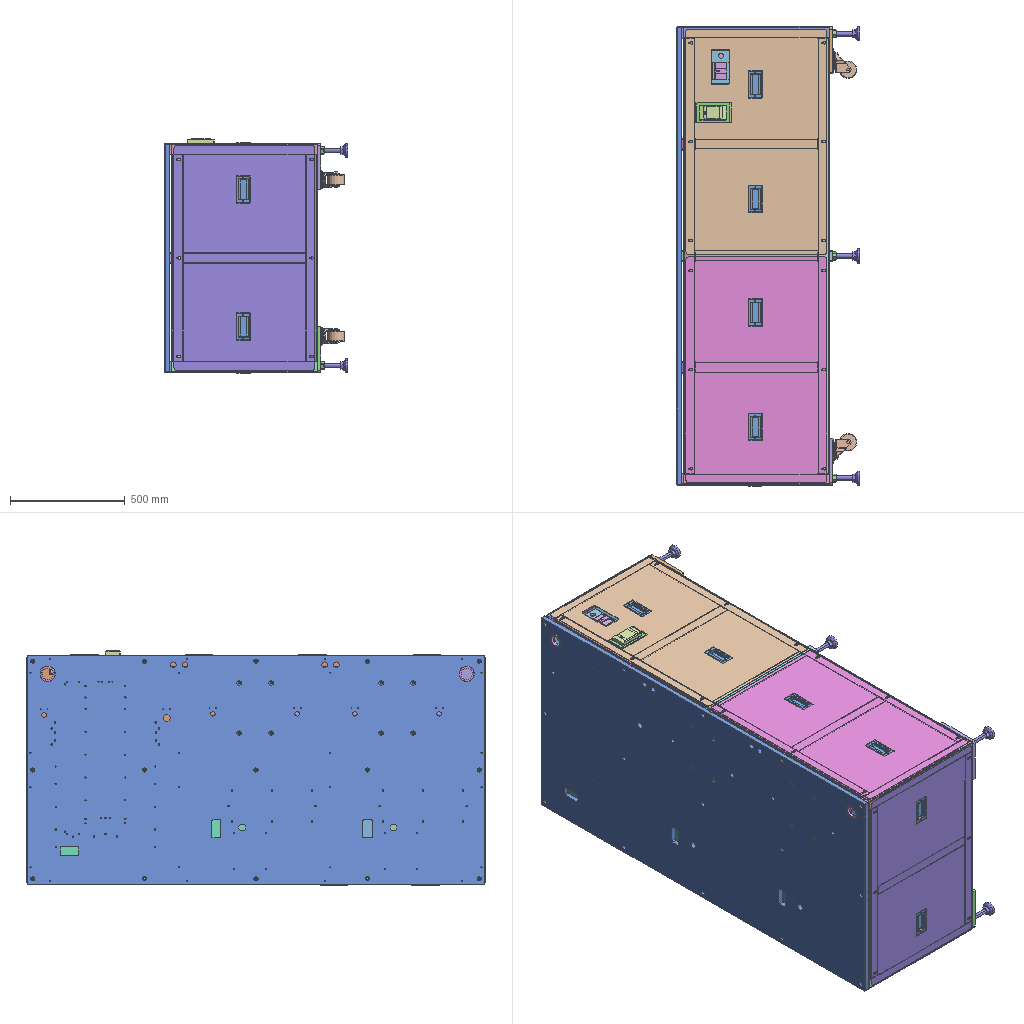Assembly | SolidWorks | 34 different items | 81 placed | box 804 x 2008 x 1025 mm
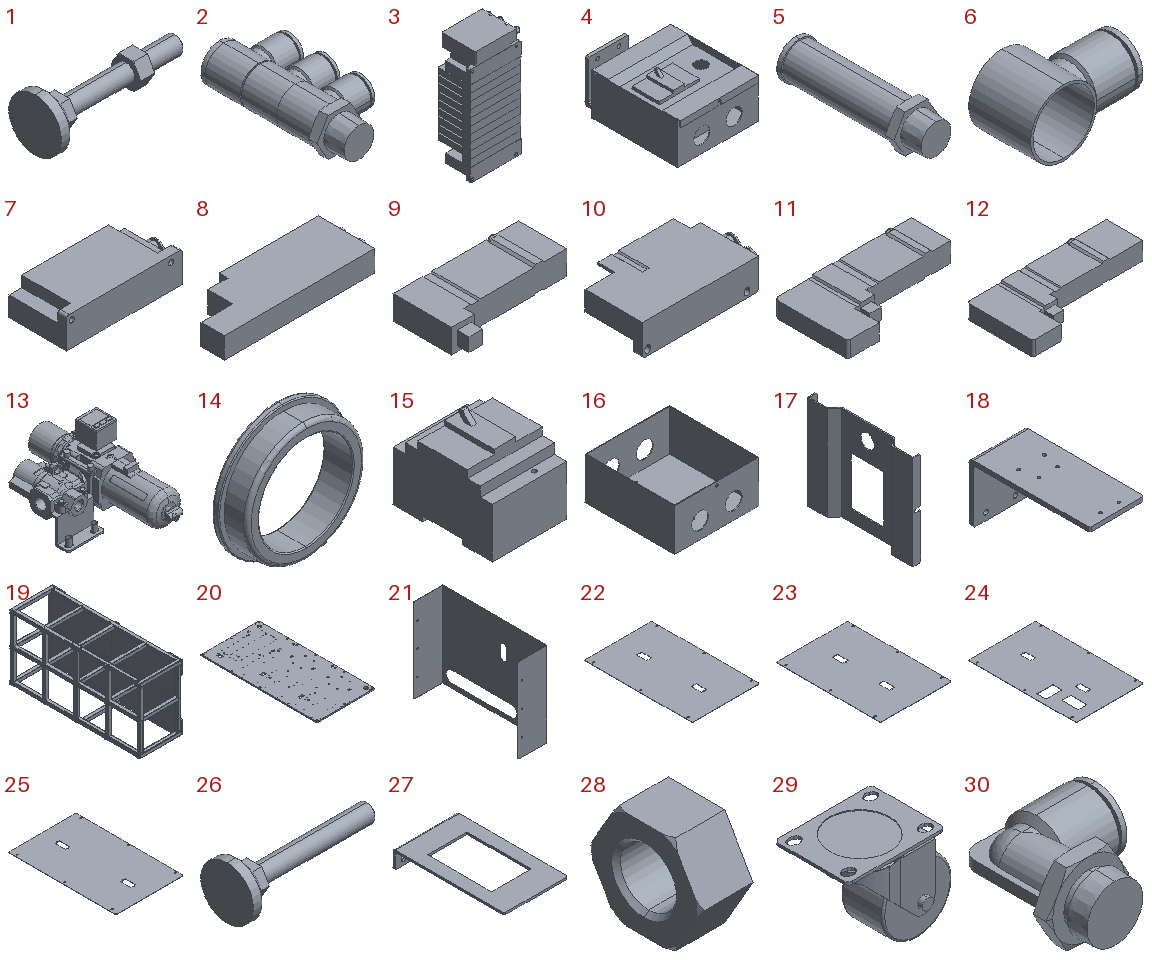Parts list (item | name | quantity | parent item | size | volume | features):
1 | (subassembly) | x6 | - | 161 x 60 x 60 mm | 104364 mm3 | -
2 | (subassembly) | x1 | - | 37.824 x 76.6 x 21 mm | 29874 mm3 | features RefAxis 3
3 | (subassembly) | x1 | - | - | 1754450 mm3 | -
4 | (subassembly) | x1 | - | 150 x 195.998 x 89.507 mm | 688254 mm3 | -
5 | - | x1 | in 2 | 24.249 x 76.6 x 21 mm | 21613 mm3 | features RefAxis 3, BaseBody 1, MoveFace 1
6 | - | x3 | in 2 | 36 x 19.2 x 20.6 mm | 2754 mm3 | features RefAxis 3, BaseBody 1
7 | - | x1 | in 3 | 121.7 x 73.2 x 30 mm | 182258 mm3 | features BaseBody 1
8 | - | x10 | in 3 | 117.6 x 42.6 x 16 mm | 66009 mm3 | features BaseBody 1
9 | - | x1 | in 3 | 78.8 x 44.194 x 18.1 mm | 37684 mm3 | features BaseBody 1
10 | - | x1 | in 3 | 121.7 x 73.2 x 30.5 mm | 162899 mm3 | features BaseBody 1
11 | - | x3 | in 3 | 103.4 x 55.58 x 18.1 mm | 53626 mm3 | features BaseBody 1
12 | - | x6 | in 3 | 116.6 x 55.58 x 18.1 mm | 59586 mm3 | features BaseBody 1
13 | - | x1 | - | - | - | features RefSurface 14, ExtruRefSurface 1
14 | - | x2 | - | 67 x 15.5 x 67 mm | 18291 mm3 | features Fillet 3, ICE 2, Extrusion 1
15 | - | x1 | in 4 | 74.7 x 99.6 x 82.007 mm | 445552 mm3 | features ICE 5, Extrusion 1, Fillet 1, HoleWzd 1
16 | - | x1 | in 4 | 150 x 163 x 75 mm | 99364 mm3 | features HoleWzd 3, ICE 2, Extrusion 1, Shell 1
17 | - | x1 | in 4 | 13.5 x 164.498 x 147 mm | 37040 mm3 | features ICE 4, Chamfer 1, ExtruThin 1, MirrorPattern 1
18 | - | x1 | in 4 | 75 x 165 x 80 mm | 106298 mm3 | features HoleWzd 3, Fillet 2, Chamfer 1, Extrusion 1, Shell 1
19 | - | x1 | - | 660 x 2000 x 1000 mm | 17994885 mm3 | features Fillet 21, HoleWzd 17, WeldCornerFeat 11, ICE 6, Chamfer 4, WeldMemberFeat 3, 3DProfileFeature 1, MoveFace 1, WeldmentFeature 1
20 | - | x1 | - | 1000 x 2000 x 20 mm | 39453468 mm3 | features HoleWzd 18, Cut 5, Chamfer 2, Extrusion 1, Fillet 1, ICE 1, MirrorPattern 1
21 | - | x1 | - | 150 x 533 x 430 mm | 664905 mm3 | features Cut 2, HoleWzd 2, Fillet 1, FlatPattern 1, ICE 1, LPattern 1, SMBaseFlange 1, SheetMetal 1
22 | - | x1 | - | 615 x 985 x 2 mm | 1193141 mm3 | features ICE 4, Extrusion 1, Fillet 1, LPattern 1
23 | - | x1 | - | 615 x 900 x 2 mm | 1088591 mm3 | features ICE 4, Extrusion 1, Fillet 1, HoleWzd 1, LPattern 1
24 | - | x1 | - | 615 x 983 x 2 mm | 1141777 mm3 | features ICE 6, Fillet 2, Extrusion 1, LPattern 1
25 | - | x2 | - | 615 x 980 x 2 mm | 1186991 mm3 | features ICE 4, Extrusion 1, Fillet 1, LPattern 1
26 | - | x6 | in 1 | 161 x 60 x 60 mm | 95763 mm3 | features RefAxis 9, 3DProfileFeature 3, ICE 1, Revolution 1
27 | - | x1 | - | 90 x 158 x 25 mm | 32642 mm3 | features Fillet 2, ICE 2, EdgeFlange 1, FlatPattern 1, SMBaseFlange 1, SheetMetal 1
28 | - | x6 | in 1 | 16 x 34.641 x 30 mm | 8601 mm3 | features RefAxis 3, 3DProfileFeature 1, ICE 1, Revolution 1
29 | - | x4 | - | 130 x 80 x 106 mm | 293823 mm3 | features ICE 12, Fillet 4, Revolution 2, Extrusion 1
30 | - | x1 | - | 33.624 x 36.35 x 21 mm | 9019 mm3 | features BaseBody 1
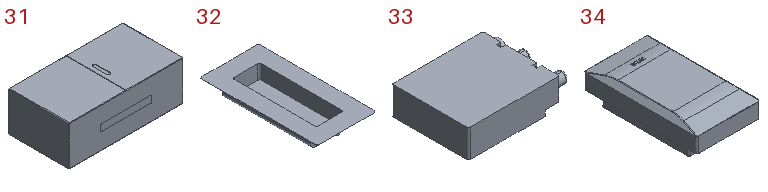31 | - | x1 | - | 1000 x 530 x 350 mm | 185406118 mm3 | features ICE 3, Fillet 2, Cut 1, Extrusion 1
32 | - | x10 | - | 60 x 120 x 15 mm | 28231 mm3 | features RefAxis 6, ICE 4, 3DProfileFeature 2, Revolution 2, Extrusion 1
33 | - | x1 | in 3 | 102.4 x 76.5 x 28.2 mm | 193130 mm3 | features BaseBody 1
34 | - | x1 | - | 65 x 116 x 32 mm | 202668 mm3 | features Fillet 5, Chamfer 3, ICE 2, Emboss 1, Extrusion 1
Mates (type | each side: item.copy, entity, surface, feature):
In the top assembly
Coincident | 19.1 face plane Boss-Extrude7 | 20.1 face plane Boss-Extrude1
Coincident | 19.1 face plane Structural Member6 | 20.1 face plane Boss-Extrude1
Concentric | 19.1 face cylinder M20 Tapped Hole1 | 26.1 face cylinder Revolve1
Coincident | 19.1 face plane Boss-Extrude2 | 28.1 face plane Revolve1
Concentric | 19.1 face cylinder M20 Tapped Hole1 | 26.2 face cylinder Revolve1
Coincident | 19.1 face plane Boss-Extrude2 | 28.2 face plane Revolve1
Concentric | 19.1 face cylinder M20 Tapped Hole2 | 26.3 face cylinder Revolve1
Coincident | 19.1 face plane Boss-Extrude25 | 28.3 face plane Revolve1
Concentric | 19.1 face cylinder M20 Tapped Hole2 | 26.4 face cylinder Revolve1
Coincident | 19.1 face plane Boss-Extrude25 | 28.4 face plane Revolve1
Concentric | 19.1 face cylinder M20 Tapped Hole1 | 26.5 face cylinder Revolve1
Coincident | 19.1 face plane Boss-Extrude2 | 28.5 face plane Revolve1
Concentric | 19.1 face cylinder M20 Tapped Hole1 | 26.6 face cylinder Revolve1
Coincident | 19.1 face plane Boss-Extrude2 | 28.6 face plane Revolve1
Concentric | 19.1 face cylinder M8 Tapped Hole1 | 29.1 face cylinder Cut-Extrude10 | 2 times
Coincident | 19.1 face plane Boss-Extrude2 | 29.1 face plane Boss-Extrude1
Concentric | 19.1 face cylinder M8 Tapped Hole1 | 29.2 face cylinder Cut-Extrude10 | 2 times
Coincident | 19.1 face plane Boss-Extrude2 | 29.2 face plane Boss-Extrude1
Concentric | 19.1 face cylinder M8 Tapped Hole1 | 29.3 face cylinder Cut-Extrude10 | 2 times
Coincident | 19.1 face plane Boss-Extrude2 | 29.3 face plane Boss-Extrude1
Concentric | 19.1 face cylinder M8 Tapped Hole1 | 29.4 face cylinder Cut-Extrude10 | 2 times
Coincident | 19.1 face plane Boss-Extrude2 | 29.4 face plane Boss-Extrude1
Coincident | 19.1 face plane Structural Member9 | 20.1 face plane Boss-Extrude1
Coincident | 19.1 face plane Structural Member5 | 25.1 face plane Boss-Extrude1
DistanceDim | 19.1 face plane Structural Member5 | 25.1 face plane Boss-Extrude1
DistanceDim | 25.1 face plane Boss-Extrude1 | 19.1 face plane Structural Member9
Coincident | 19.1 face plane Structural Member6 | 21.1 face plane Base-Flange1
DistanceDim | 21.1 face plane Base-Flange1 | 19.1 face plane Structural Member6
Coincident | 19.1 face plane Structural Member6 | 18.1 face plane Boss-Extrude1
DistanceDim | 17.1 face plane Extrude-Thin1 | 19.1 face plane Structural Member6
Coincident | 19.1 face plane Structural Member5 | 22.1 face plane Boss-Extrude1
DistanceDim | 19.1 face plane Structural Member5 | 22.1 face plane Boss-Extrude1
DistanceDim | 19.1 face plane Structural Member6 | 22.1 face plane Boss-Extrude1
Coincident | 19.1 face plane Structural Member5 | 24.1 face plane Boss-Extrude1
DistanceDim | 19.1 face plane Structural Member6 | 24.1 face plane Boss-Extrude1
DistanceDim | 19.1 face plane Structural Member5 | 24.1 face plane Boss-Extrude1
Coincident | 19.1 face plane Structural Member5 | 23.1 face plane Boss-Extrude1
DistanceDim | 19.1 face plane Structural Member5 | 23.1 face plane Boss-Extrude1
DistanceDim | 23.1 face plane Boss-Extrude1 | 19.1 face plane Structural Member6
DistanceDim | 19.1 face plane Structural Member5 | 21.1 face plane Base-Flange1
Coincident | 19.1 face plane Structural Member6 | 31.1 face plane Boss-Extrude1
DistanceDim | 31.1 face plane Boss-Extrude1 | 19.1 face plane Structural Member5
DistanceDim | 31.1 face plane Boss-Extrude1 | 19.1 face plane Structural Member6
DistanceDim | 16.1 face plane Boss-Extrude1 | 19.1 face plane Structural Member5
Coincident | 19.1 face plane Structural Member6 | 27.1 face plane Edge-Flange1
Coincident | 19.1 face plane Structural Member6 | 27.1 face plane Base-Flange1
DistanceDim | 27.1 face plane Edge-Flange1 | 16.1 face plane Boss-Extrude1
Coincident | 27.1 face plane Base-Flange1 | 34.1 face plane Boss-Extrude2
Coincident | 27.1 face plane Cut-Extrude2 | 34.1 face plane Boss-Extrude1 | 2 times
Coincident | 20.1 face plane Boss-Extrude1 | 14.1 face plane Boss-Extrude2
Coincident | 20.1 face plane Boss-Extrude1 | 14.2 face plane Boss-Extrude2
Concentric | 20.1 face cylinder Cut-Extrude1 | 14.1 face cylinder Boss-Extrude1
Concentric | 20.1 face cylinder Cut-Extrude1 | 14.2 face cylinder Boss-Extrude1
Coincident | 22.1 face plane Boss-Extrude1 | 32.1 face plane Boss-Extrude2
Coincident | 32.2 face plane Boss-Extrude2 | 32.1 face plane Boss-Extrude2
Concentric | 22.1 face cylinder Cut-Extrude5 | 32.1 face cylinder Revolve2
Concentric | 22.1 face cylinder Cut-Extrude5 | 32.1 face cylinder Revolve1
Concentric | 22.1 face cylinder Cut-Extrude5 | 32.2 face cylinder Revolve2
Concentric | 22.1 face cylinder Cut-Extrude5 | 32.2 face cylinder Revolve1
Coincident | 24.1 face plane Boss-Extrude1 | 32.3 face plane Boss-Extrude2
Coincident | 32.3 face plane Boss-Extrude2 | 32.4 face plane Boss-Extrude2
Concentric | 24.1 face cylinder Cut-Extrude5 | 32.3 face cylinder Revolve1
Concentric | 24.1 face cylinder Cut-Extrude5 | 32.3 face cylinder Revolve2
Concentric | 24.1 face cylinder Cut-Extrude5 | 32.4 face cylinder Revolve1
Concentric | 24.1 face cylinder Cut-Extrude5 | 32.4 face cylinder Revolve2
Coincident | 25.1 face plane Boss-Extrude1 | 32.5 face plane Boss-Extrude2
Coincident | 32.6 face plane Boss-Extrude2 | 32.5 face plane Boss-Extrude2
Concentric | 25.1 face cylinder Cut-Extrude5 | 32.5 face cylinder Revolve1
Concentric | 25.1 face cylinder Cut-Extrude5 | 32.5 face cylinder Revolve2
Concentric | 25.1 face cylinder Cut-Extrude5 | 32.6 face cylinder Revolve1
Concentric | 25.1 face cylinder Cut-Extrude5 | 32.6 face cylinder Revolve2
Coincident | 23.1 face plane Boss-Extrude1 | 32.7 face plane Boss-Extrude2
Coincident | 23.1 face plane Boss-Extrude1 | 32.8 face plane Boss-Extrude2
Concentric | 23.1 face cylinder Cut-Extrude5 | 32.8 face cylinder Revolve1
Concentric | 23.1 face cylinder Cut-Extrude5 | 32.8 face cylinder Revolve2
Concentric | 23.1 face cylinder Cut-Extrude5 | 32.7 face cylinder Revolve1
Concentric | 23.1 face cylinder Cut-Extrude5 | 32.7 face cylinder Revolve2
Coincident | 21.1 face plane Base-Flange1 | 7.1 face plane Input1
Concentric | 21.1 face cylinder M4 Tapped Hole1 | 7.1 face cylinder Input1 | 2 times
Coincident | 25.2 face plane Boss-Extrude1 | 32.9 face plane Boss-Extrude2
Concentric | 30.1 face cone Input1 | 13.1 face cylinder VHS30-03A-B-1/1_1-1-surface2
Coincident | 30.1 face plane Input1 | 13.1 face plane VHS30-03A-B-1/1_1-1-surface2
Concentric | 5.1 face cone Input1 | 13.1 face cylinder AW30-03B-1/1-1-surface1
Coincident | 5.1 face plane Input1 | 13.1 face plane AW30-03B-1/1-1-surface1
Coincident | 21.1 face plane Base-Flange1 | 13.1 face plane AW30-03B-1/4-1-surface1
Coincident | 21.1 face plane Base-Flange1 | 13.1 face plane VHS30-03A-B-1/1_1-1-surface2
DistanceDim | 13.1 face plane AW30-03B-1/4-1-surface1 | 21.1 face plane Base-Flange1
In subassembly 2
Concentric | 5.2 face cylinder Input1 | 6.1 face cylinder Input1
Coincident | 5.2 face plane Input1 | 6.1 face plane Input1
In subassembly 4
Coincident | 16.2 face plane Boss-Extrude1 | 17.2 face plane Extrude-Thin1 | 2 times
Coincident | 16.2 face plane Shell1 | 17.2 face plane Extrude-Thin1
Concentric | 16.2 face cylinder Ø5.5 (5.5) Diameter Hole1 | 18.2 face cylinder M5 Tapped Hole1 | 2 times
Coincident | 16.2 face plane Boss-Extrude1 | 18.2 face plane Shell1
Concentric | 18.2 face cylinder M4 Tapped Hole1 | 15.1 face cylinder Ø4.5 (4.5) Diameter Hole1 | 2 times
Coincident | 16.2 face plane Shell1 | 15.1 face plane Boss-Extrude1
In subassembly 3
Coincident | 11.1 face plane Input1 | 11.2 face plane Input1
Coincident | 8.1 face plane Input1 | 11.2 face plane Input1
Coincident | 12.1 face plane Input1 | 8.2 face plane Input1
Coincident | 12.1 face plane Input1 | 12.2 face plane Input1
In subassembly 1
Coincident | 26.7 axis | 28.7 axis
Coincident | 26.7 face plane Cut-Extrude1 | 28.7 face plane Cut-Extrude1
DistanceDim | 28.7 face plane Revolve1 | 26.7 face plane Revolve1